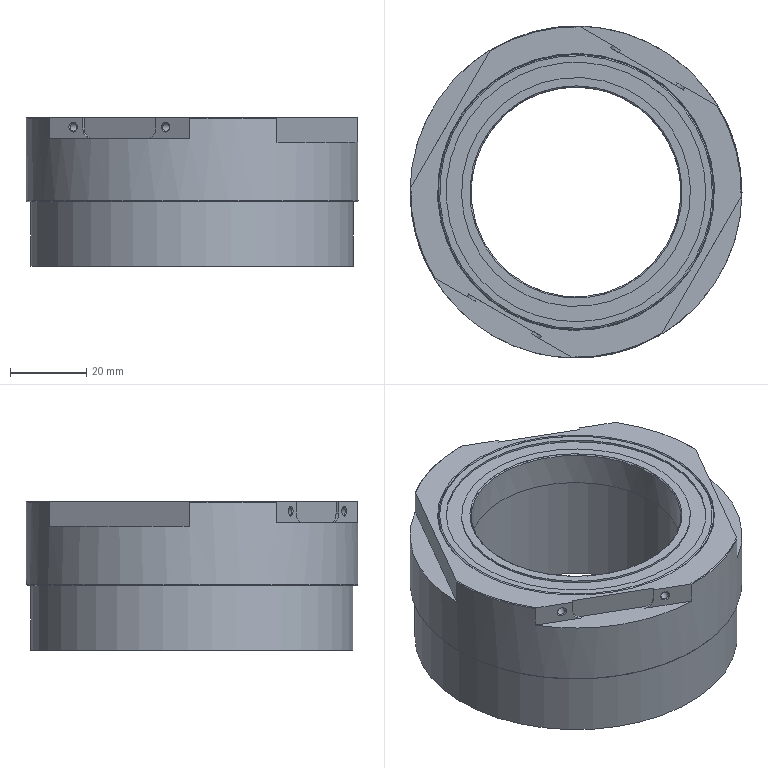Part | STEP file | 1 solid | 54 faces | box 87 x 87 x 39 mm | volume 122387 mm3 | plane 23 | cylinder 19 | cone 10 | torus 2 | commonest cylinder face diameters 72.1 x5 2.05 x4 5 x4 55 x1 57.5 x1 60 x1